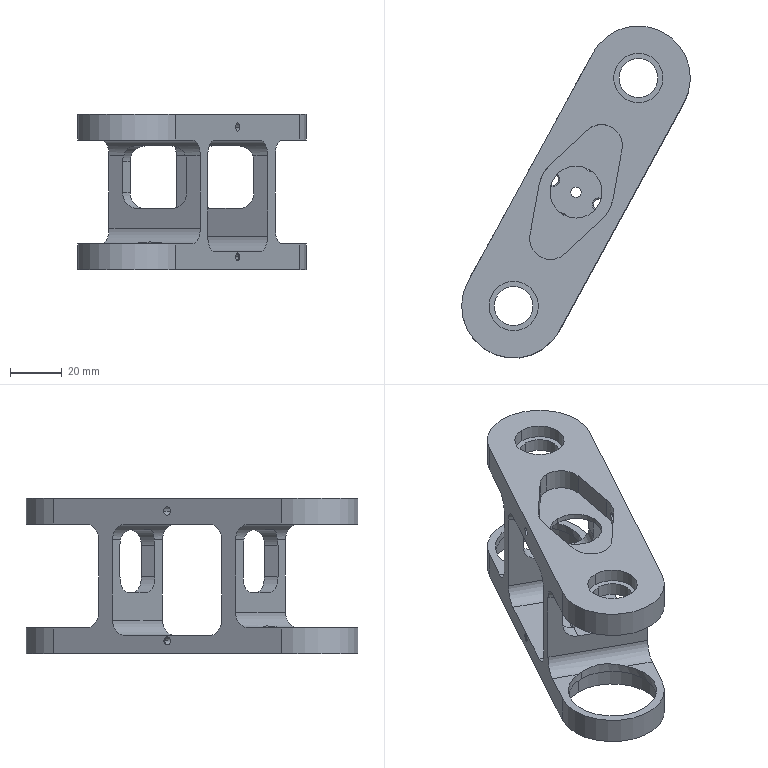Part | SolidWorks | features BaseBody 1 | 1 solid | 139 faces | box 87.991 x 127.732 x 60 mm | volume 76857 mm3 | cylinder 73 | plane 40 | cone 26 | commonest cylinder face diameters 12 x16 2.5 x8 4.2 x8 40 x6 3.2 x4 6 x4